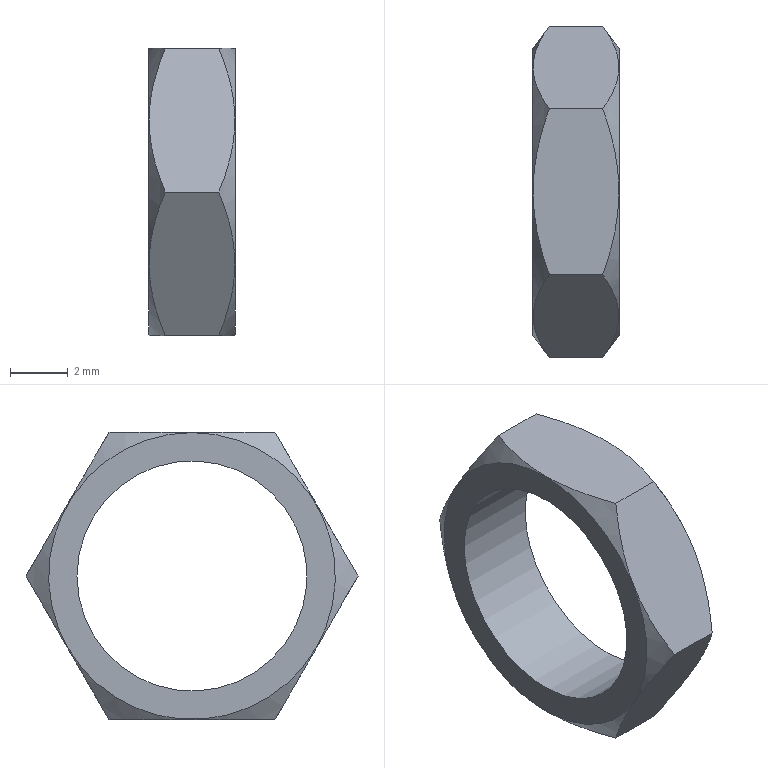Part | STEP file | 1-43.15 | 1 solid | 11 faces | box 3 x 11.547 x 10 mm | volume 106.106 mm3 | plane 8 | cone 2 | cylinder 1 | commonest cylinder face diameters 8 x1
STEP:
#1=CARTESIAN_POINT('',(0.,0.,0.));
#2=DIRECTION('',(0.,0.,1.));
#3=DIRECTION('',(1.,0.,0.));
#4=AXIS2_PLACEMENT_3D('',#1,#2,#3);
#5=CARTESIAN_POINT('',(1.5,4.,0.));
#6=VERTEX_POINT('',#5);
#7=CARTESIAN_POINT('',(1.5,0.,0.));
#8=DIRECTION('',(-1.,0.,0.));
#9=DIRECTION('',(0.,1.,0.));
#10=AXIS2_PLACEMENT_3D('',#7,#8,#9);
#11=CIRCLE('',#10,4.);
#12=CARTESIAN_POINT('',(1.5,0.,0.));
#13=DIRECTION('',(-1.,0.,0.));
#14=DIRECTION('',(0.,1.,0.));
#15=AXIS2_PLACEMENT_3D('',#12,#13,#14);
#16=CYLINDRICAL_SURFACE('',#15,4.);
#17=CARTESIAN_POINT('',(0.,0.));
#18=DIRECTION('',(1.,0.));
#19=VECTOR('',#18,1.);
#20=LINE('',#17,#19);
#21=(GEOMETRIC_REPRESENTATION_CONTEXT(2)PARAMETRIC_REPRESENTATION_CONTEXT()REPRESENTATION_CONTEXT('',''));
#22=DEFINITIONAL_REPRESENTATION('',(#20),#21);
#23=PCURVE('',#16,#22);
#24=CARTESIAN_POINT('',(1.5,0.,0.7735));
#25=DIRECTION('',(1.,0.,0.));
#26=DIRECTION('',(0.,1.,0.));
#27=AXIS2_PLACEMENT_3D('',#24,#25,#26);
#28=PLANE('',#27);
#29=CARTESIAN_POINT('',(4.,-0.7735));
#30=CARTESIAN_POINT('',(4.,-7.702));
#31=CARTESIAN_POINT('',(-2.,-4.238));
#32=CARTESIAN_POINT('',(-8.,-0.7735));
#33=CARTESIAN_POINT('',(-2.,2.691));
#34=CARTESIAN_POINT('',(4.,6.155));
#35=CARTESIAN_POINT('',(4.,-0.7735));
#36=(BOUNDED_CURVE()B_SPLINE_CURVE(2,(#29,#30,#31,#32,#33,#34,#35),.UNSPECIFIED.,.T.,.F.)B_SPLINE_CURVE_WITH_KNOTS((1,2,2,2,2,1),(-2.094,0.,2.094,4.189,6.283,8.378),.UNSPECIFIED.)CURVE()GEOMETRIC_REPRESENTATION_ITEM()RATIONAL_B_SPLINE_CURVE((1.,0.5,1.,0.5,1.,0.5,1.))REPRESENTATION_ITEM(''));
#37=(GEOMETRIC_REPRESENTATION_CONTEXT(2)PARAMETRIC_REPRESENTATION_CONTEXT()REPRESENTATION_CONTEXT('',''));
#38=DEFINITIONAL_REPRESENTATION('',(#36),#37);
#39=PCURVE('',#28,#38);
#40=SURFACE_CURVE('',#11,(#23,#39),.PCURVE_S1.);
#41=EDGE_CURVE('',#6,#6,#40,.T.);
#42=ORIENTED_EDGE('',*,*,#41,.T.);
#43=CARTESIAN_POINT('',(-1.5,4.,0.));
#44=VERTEX_POINT('',#43);
#45=CARTESIAN_POINT('',(1.5,4.,0.));
#46=DIRECTION('',(-1.,0.,0.));
#47=VECTOR('',#46,1.);
#48=LINE('',#45,#47);
#49=CARTESIAN_POINT('',(6.283,0.));
#50=DIRECTION('',(0.,1.));
#51=VECTOR('',#50,1.);
#52=LINE('',#49,#51);
#53=(GEOMETRIC_REPRESENTATION_CONTEXT(2)PARAMETRIC_REPRESENTATION_CONTEXT()REPRESENTATION_CONTEXT('',''));
#54=DEFINITIONAL_REPRESENTATION('',(#52),#53);
#55=PCURVE('',#16,#54);
#56=CARTESIAN_POINT('',(0.,0.));
#57=DIRECTION('',(0.,1.));
#58=VECTOR('',#57,1.);
#59=LINE('',#56,#58);
#60=(GEOMETRIC_REPRESENTATION_CONTEXT(2)PARAMETRIC_REPRESENTATION_CONTEXT()REPRESENTATION_CONTEXT('',''));
#61=DEFINITIONAL_REPRESENTATION('',(#59),#60);
#62=PCURVE('',#16,#61);
#63=SEAM_CURVE('',#48,(#55,#62),.PCURVE_S1.);
#64=EDGE_CURVE('',#6,#44,#63,.T.);
#65=ORIENTED_EDGE('',*,*,#64,.T.);
#66=CARTESIAN_POINT('',(-1.5,0.,0.));
#67=DIRECTION('',(-1.,0.,0.));
#68=DIRECTION('',(0.,1.,0.));
#69=AXIS2_PLACEMENT_3D('',#66,#67,#68);
#70=CIRCLE('',#69,4.);
#71=CARTESIAN_POINT('',(0.,3.));
#72=DIRECTION('',(1.,0.));
#73=VECTOR('',#72,1.);
#74=LINE('',#71,#73);
#75=(GEOMETRIC_REPRESENTATION_CONTEXT(2)PARAMETRIC_REPRESENTATION_CONTEXT()REPRESENTATION_CONTEXT('',''));
#76=DEFINITIONAL_REPRESENTATION('',(#74),#75);
#77=PCURVE('',#16,#76);
#78=CARTESIAN_POINT('',(-1.5,0.,0.7735));
#79=DIRECTION('',(1.,0.,0.));
#80=DIRECTION('',(0.,1.,0.));
#81=AXIS2_PLACEMENT_3D('',#78,#79,#80);
#82=PLANE('',#81);
#83=CARTESIAN_POINT('',(4.,-0.7735));
#84=CARTESIAN_POINT('',(4.,-7.702));
#85=CARTESIAN_POINT('',(-2.,-4.238));
#86=CARTESIAN_POINT('',(-8.,-0.7735));
#87=CARTESIAN_POINT('',(-2.,2.691));
#88=CARTESIAN_POINT('',(4.,6.155));
#89=CARTESIAN_POINT('',(4.,-0.7735));
#90=(BOUNDED_CURVE()B_SPLINE_CURVE(2,(#83,#84,#85,#86,#87,#88,#89),.UNSPECIFIED.,.T.,.F.)B_SPLINE_CURVE_WITH_KNOTS((1,2,2,2,2,1),(-2.094,0.,2.094,4.189,6.283,8.378),.UNSPECIFIED.)CURVE()GEOMETRIC_REPRESENTATION_ITEM()RATIONAL_B_SPLINE_CURVE((1.,0.5,1.,0.5,1.,0.5,1.))REPRESENTATION_ITEM(''));
#91=(GEOMETRIC_REPRESENTATION_CONTEXT(2)PARAMETRIC_REPRESENTATION_CONTEXT()REPRESENTATION_CONTEXT('',''));
#92=DEFINITIONAL_REPRESENTATION('',(#90),#91);
#93=PCURVE('',#82,#92);
#94=SURFACE_CURVE('',#70,(#77,#93),.PCURVE_S1.);
#95=EDGE_CURVE('',#44,#44,#94,.T.);
#96=ORIENTED_EDGE('',*,*,#95,.F.);
#97=ORIENTED_EDGE('',*,*,#64,.F.);
#98=EDGE_LOOP('',(#42,#65,#96,#97));
#99=FACE_BOUND('',#98,.F.);
#100=ADVANCED_FACE('',(#99),#16,.F.);
#101=CARTESIAN_POINT('',(1.5,0.,4.986));
#102=VERTEX_POINT('',#101);
#103=CARTESIAN_POINT('',(1.5,0.,0.));
#104=DIRECTION('',(1.,0.,0.));
#105=DIRECTION('',(0.,0.,1.));
#106=AXIS2_PLACEMENT_3D('',#103,#104,#105);
#107=CIRCLE('',#106,4.986);
#108=CARTESIAN_POINT('',(0.,-0.7735));
#109=DIRECTION('',(0.,1.));
#110=AXIS2_PLACEMENT_2D('',#108,#109);
#111=CIRCLE('',#110,4.986);
#112=(GEOMETRIC_REPRESENTATION_CONTEXT(2)PARAMETRIC_REPRESENTATION_CONTEXT()REPRESENTATION_CONTEXT('',''));
#113=DEFINITIONAL_REPRESENTATION('',(#111),#112);
#114=PCURVE('',#28,#113);
#115=CARTESIAN_POINT('',(1.5,0.,0.));
#116=DIRECTION('',(-1.,0.,0.));
#117=DIRECTION('',(0.,0.,1.));
#118=AXIS2_PLACEMENT_3D('',#115,#116,#117);
#119=CONICAL_SURFACE('',#118,4.986,0.9416);
#120=CARTESIAN_POINT('',(6.283,0.));
#121=DIRECTION('',(-1.,0.));
#122=VECTOR('',#121,1.);
#123=LINE('',#120,#122);
#124=(GEOMETRIC_REPRESENTATION_CONTEXT(2)PARAMETRIC_REPRESENTATION_CONTEXT()REPRESENTATION_CONTEXT('',''));
#125=DEFINITIONAL_REPRESENTATION('',(#123),#124);
#126=PCURVE('',#119,#125);
#127=SURFACE_CURVE('',#107,(#114,#126),.PCURVE_S1.);
#128=EDGE_CURVE('',#102,#102,#127,.T.);
#129=ORIENTED_EDGE('',*,*,#128,.T.);
#130=EDGE_LOOP('',(#129));
#131=FACE_BOUND('',#130,.T.);
#132=ORIENTED_EDGE('',*,*,#41,.T.);
#133=EDGE_LOOP('',(#132));
#134=FACE_BOUND('',#133,.T.);
#135=ADVANCED_FACE('',(#131,#134),#28,.T.);
#136=CARTESIAN_POINT('',(-1.5,0.,4.986));
#137=VERTEX_POINT('',#136);
#138=CARTESIAN_POINT('',(-1.5,0.,0.));
#139=DIRECTION('',(1.,0.,0.));
#140=DIRECTION('',(0.,0.,1.));
#141=AXIS2_PLACEMENT_3D('',#138,#139,#140);
#142=CIRCLE('',#141,4.986);
#143=CARTESIAN_POINT('',(0.,-0.7735));
#144=DIRECTION('',(0.,1.));
#145=AXIS2_PLACEMENT_2D('',#143,#144);
#146=CIRCLE('',#145,4.986);
#147=(GEOMETRIC_REPRESENTATION_CONTEXT(2)PARAMETRIC_REPRESENTATION_CONTEXT()REPRESENTATION_CONTEXT('',''));
#148=DEFINITIONAL_REPRESENTATION('',(#146),#147);
#149=PCURVE('',#82,#148);
#150=CARTESIAN_POINT('',(-1.5,0.,0.));
#151=DIRECTION('',(1.,0.,0.));
#152=DIRECTION('',(0.,0.,1.));
#153=AXIS2_PLACEMENT_3D('',#150,#151,#152);
#154=CONICAL_SURFACE('',#153,4.986,0.9416);
#155=CARTESIAN_POINT('',(0.,0.));
#156=DIRECTION('',(1.,0.));
#157=VECTOR('',#156,1.);
#158=LINE('',#155,#157);
#159=(GEOMETRIC_REPRESENTATION_CONTEXT(2)PARAMETRIC_REPRESENTATION_CONTEXT()REPRESENTATION_CONTEXT('',''));
#160=DEFINITIONAL_REPRESENTATION('',(#158),#159);
#161=PCURVE('',#154,#160);
#162=SURFACE_CURVE('',#142,(#149,#161),.PCURVE_S1.);
#163=EDGE_CURVE('',#137,#137,#162,.T.);
#164=ORIENTED_EDGE('',*,*,#163,.T.);
#165=EDGE_LOOP('',(#164));
#166=FACE_BOUND('',#165,.F.);
#167=ORIENTED_EDGE('',*,*,#95,.T.);
#168=EDGE_LOOP('',(#167));
#169=FACE_BOUND('',#168,.F.);
#170=ADVANCED_FACE('',(#166,#169),#82,.F.);
#171=CARTESIAN_POINT('',(0.9268,5.774,0.));
#172=VERTEX_POINT('',#171);
#173=CARTESIAN_POINT('',(-0.9268,5.774,0.));
#174=VERTEX_POINT('',#173);
#175=CARTESIAN_POINT('',(0.9268,5.774,0.));
#176=DIRECTION('',(-1.,0.,0.));
#177=VECTOR('',#176,1.);
#178=LINE('',#175,#177);
#179=CARTESIAN_POINT('',(0.,4.33,2.5));
#180=DIRECTION('',(0.,-0.866,-0.5));
#181=DIRECTION('',(0.,-0.5,0.866));
#182=AXIS2_PLACEMENT_3D('',#179,#180,#181);
#183=PLANE('',#182);
#184=CARTESIAN_POINT('',(-2.887,-0.9268));
#185=DIRECTION('',(0.,1.));
#186=VECTOR('',#185,1.);
#187=LINE('',#184,#186);
#188=(GEOMETRIC_REPRESENTATION_CONTEXT(2)PARAMETRIC_REPRESENTATION_CONTEXT()REPRESENTATION_CONTEXT('',''));
#189=DEFINITIONAL_REPRESENTATION('',(#187),#188);
#190=PCURVE('',#183,#189);
#191=CARTESIAN_POINT('',(0.,4.33,-2.5));
#192=DIRECTION('',(0.,-0.866,0.5));
#193=DIRECTION('',(0.,0.5,0.866));
#194=AXIS2_PLACEMENT_3D('',#191,#192,#193);
#195=PLANE('',#194);
#196=CARTESIAN_POINT('',(2.887,-0.9268));
#197=DIRECTION('',(0.,1.));
#198=VECTOR('',#197,1.);
#199=LINE('',#196,#198);
#200=(GEOMETRIC_REPRESENTATION_CONTEXT(2)PARAMETRIC_REPRESENTATION_CONTEXT()REPRESENTATION_CONTEXT('',''));
#201=DEFINITIONAL_REPRESENTATION('',(#199),#200);
#202=PCURVE('',#195,#201);
#203=SURFACE_CURVE('',#178,(#190,#202),.PCURVE_S1.);
#204=EDGE_CURVE('',#172,#174,#203,.T.);
#205=ORIENTED_EDGE('',*,*,#204,.F.);
#206=CARTESIAN_POINT('',(0.9268,2.887,5.));
#207=VERTEX_POINT('',#206);
#208=CARTESIAN_POINT('',(0.9268,5.774,0.));
#209=CARTESIAN_POINT('',(1.977,4.33,2.5));
#210=CARTESIAN_POINT('',(0.9268,2.887,5.));
#211=(BOUNDED_CURVE()B_SPLINE_CURVE(2,(#208,#209,#210),.UNSPECIFIED.,.F.,.F.)B_SPLINE_CURVE_WITH_KNOTS((3,3),(0.,1.),.PIECEWISE_BEZIER_KNOTS.)CURVE()GEOMETRIC_REPRESENTATION_ITEM()RATIONAL_B_SPLINE_CURVE((1.118,1.291,1.118))REPRESENTATION_ITEM(''));
#212=CARTESIAN_POINT('',(-2.887,-0.9268));
#213=CARTESIAN_POINT('',(0.,-1.977));
#214=CARTESIAN_POINT('',(2.887,-0.9268));
#215=(BOUNDED_CURVE()B_SPLINE_CURVE(2,(#212,#213,#214),.UNSPECIFIED.,.F.,.F.)B_SPLINE_CURVE_WITH_KNOTS((3,3),(0.,1.),.PIECEWISE_BEZIER_KNOTS.)CURVE()GEOMETRIC_REPRESENTATION_ITEM()RATIONAL_B_SPLINE_CURVE((1.118,1.291,1.118))REPRESENTATION_ITEM(''));
#216=(GEOMETRIC_REPRESENTATION_CONTEXT(2)PARAMETRIC_REPRESENTATION_CONTEXT()REPRESENTATION_CONTEXT('',''));
#217=DEFINITIONAL_REPRESENTATION('',(#215),#216);
#218=PCURVE('',#183,#217);
#219=CARTESIAN_POINT('',(1.571,0.5732));
#220=CARTESIAN_POINT('',(1.556,0.5365));
#221=CARTESIAN_POINT('',(1.525,0.4673));
#222=CARTESIAN_POINT('',(1.479,0.3758));
#223=CARTESIAN_POINT('',(1.432,0.2957));
#224=CARTESIAN_POINT('',(1.385,0.2264));
#225=CARTESIAN_POINT('',(1.338,0.1674));
#226=CARTESIAN_POINT('',(1.29,0.1182));
#227=CARTESIAN_POINT('',(1.241,0.0784));
#228=CARTESIAN_POINT('',(1.193,0.04775));
#229=CARTESIAN_POINT('',(1.145,0.02601));
#230=CARTESIAN_POINT('',(1.096,0.01303));
#231=CARTESIAN_POINT('',(1.047,0.008712));
#232=CARTESIAN_POINT('',(0.9985,0.01303));
#233=CARTESIAN_POINT('',(0.9498,0.02601));
#234=CARTESIAN_POINT('',(0.9013,0.04775));
#235=CARTESIAN_POINT('',(0.8529,0.0784));
#236=CARTESIAN_POINT('',(0.8048,0.1182));
#237=CARTESIAN_POINT('',(0.7569,0.1674));
#238=CARTESIAN_POINT('',(0.7094,0.2264));
#239=CARTESIAN_POINT('',(0.6622,0.2957));
#240=CARTESIAN_POINT('',(0.6155,0.3758));
#241=CARTESIAN_POINT('',(0.5692,0.4673));
#242=CARTESIAN_POINT('',(0.5388,0.5365));
#243=CARTESIAN_POINT('',(0.5236,0.5732));
#244=B_SPLINE_CURVE_WITH_KNOTS('',3,(#219,#220,#221,#222,#223,#224,#225,#226,#227,#228,#229,#230,#231,#232,#233,#234,#235,#236,#237,#238,#239,#240,#241,#242,#243),.UNSPECIFIED.,.F.,.F.,(4,1,1,1,1,1,1,1,1,1,1,1,1,1,1,1,1,1,1,1,1,1,4),(0.,0.04545,0.09091,0.1364,0.1818,0.2273,0.2727,0.3182,0.3636,0.4091,0.4545,0.5,0.5455,0.5909,0.6364,0.6818,0.7273,0.7727,0.8182,0.8636,0.9091,0.9545,1.),.QUASI_UNIFORM_KNOTS.);
#245=(GEOMETRIC_REPRESENTATION_CONTEXT(2)PARAMETRIC_REPRESENTATION_CONTEXT()REPRESENTATION_CONTEXT('',''));
#246=DEFINITIONAL_REPRESENTATION('',(#244),#245);
#247=PCURVE('',#119,#246);
#248=SURFACE_CURVE('',#211,(#218,#247),.PCURVE_S1.);
#249=EDGE_CURVE('',#172,#207,#248,.T.);
#250=ORIENTED_EDGE('',*,*,#249,.T.);
#251=CARTESIAN_POINT('',(-0.9268,2.887,5.));
#252=VERTEX_POINT('',#251);
#253=CARTESIAN_POINT('',(0.9268,2.887,5.));
#254=DIRECTION('',(-1.,0.,0.));
#255=VECTOR('',#254,1.);
#256=LINE('',#253,#255);
#257=CARTESIAN_POINT('',(2.887,-0.9268));
#258=DIRECTION('',(0.,1.));
#259=VECTOR('',#258,1.);
#260=LINE('',#257,#259);
#261=(GEOMETRIC_REPRESENTATION_CONTEXT(2)PARAMETRIC_REPRESENTATION_CONTEXT()REPRESENTATION_CONTEXT('',''));
#262=DEFINITIONAL_REPRESENTATION('',(#260),#261);
#263=PCURVE('',#183,#262);
#264=CARTESIAN_POINT('',(0.,0.,5.));
#265=DIRECTION('',(0.,0.,-1.));
#266=DIRECTION('',(0.,-1.,0.));
#267=AXIS2_PLACEMENT_3D('',#264,#265,#266);
#268=PLANE('',#267);
#269=CARTESIAN_POINT('',(-2.887,-0.9268));
#270=DIRECTION('',(0.,1.));
#271=VECTOR('',#270,1.);
#272=LINE('',#269,#271);
#273=(GEOMETRIC_REPRESENTATION_CONTEXT(2)PARAMETRIC_REPRESENTATION_CONTEXT()REPRESENTATION_CONTEXT('',''));
#274=DEFINITIONAL_REPRESENTATION('',(#272),#273);
#275=PCURVE('',#268,#274);
#276=SURFACE_CURVE('',#256,(#263,#275),.PCURVE_S1.);
#277=EDGE_CURVE('',#207,#252,#276,.T.);
#278=ORIENTED_EDGE('',*,*,#277,.T.);
#279=CARTESIAN_POINT('',(-0.9268,2.887,5.));
#280=CARTESIAN_POINT('',(-1.977,4.33,2.5));
#281=CARTESIAN_POINT('',(-0.9268,5.774,0.));
#282=(BOUNDED_CURVE()B_SPLINE_CURVE(2,(#279,#280,#281),.UNSPECIFIED.,.F.,.F.)B_SPLINE_CURVE_WITH_KNOTS((3,3),(0.,1.),.PIECEWISE_BEZIER_KNOTS.)CURVE()GEOMETRIC_REPRESENTATION_ITEM()RATIONAL_B_SPLINE_CURVE((1.118,1.291,1.118))REPRESENTATION_ITEM(''));
#283=CARTESIAN_POINT('',(2.887,0.9268));
#284=CARTESIAN_POINT('',(0.,1.977));
#285=CARTESIAN_POINT('',(-2.887,0.9268));
#286=(BOUNDED_CURVE()B_SPLINE_CURVE(2,(#283,#284,#285),.UNSPECIFIED.,.F.,.F.)B_SPLINE_CURVE_WITH_KNOTS((3,3),(0.,1.),.PIECEWISE_BEZIER_KNOTS.)CURVE()GEOMETRIC_REPRESENTATION_ITEM()RATIONAL_B_SPLINE_CURVE((1.118,1.291,1.118))REPRESENTATION_ITEM(''));
#287=(GEOMETRIC_REPRESENTATION_CONTEXT(2)PARAMETRIC_REPRESENTATION_CONTEXT()REPRESENTATION_CONTEXT('',''));
#288=DEFINITIONAL_REPRESENTATION('',(#286),#287);
#289=PCURVE('',#183,#288);
#290=CARTESIAN_POINT('',(5.76,0.5732));
#291=CARTESIAN_POINT('',(5.744,0.5365));
#292=CARTESIAN_POINT('',(5.714,0.4673));
#293=CARTESIAN_POINT('',(5.668,0.3758));
#294=CARTESIAN_POINT('',(5.621,0.2957));
#295=CARTESIAN_POINT('',(5.574,0.2264));
#296=CARTESIAN_POINT('',(5.526,0.1674));
#297=CARTESIAN_POINT('',(5.478,0.1182));
#298=CARTESIAN_POINT('',(5.43,0.0784));
#299=CARTESIAN_POINT('',(5.382,0.04775));
#300=CARTESIAN_POINT('',(5.333,0.02601));
#301=CARTESIAN_POINT('',(5.285,0.01303));
#302=CARTESIAN_POINT('',(5.236,0.008712));
#303=CARTESIAN_POINT('',(5.187,0.01303));
#304=CARTESIAN_POINT('',(5.139,0.02601));
#305=CARTESIAN_POINT('',(5.09,0.04775));
#306=CARTESIAN_POINT('',(5.042,0.0784));
#307=CARTESIAN_POINT('',(4.994,0.1182));
#308=CARTESIAN_POINT('',(4.946,0.1674));
#309=CARTESIAN_POINT('',(4.898,0.2264));
#310=CARTESIAN_POINT('',(4.851,0.2957));
#311=CARTESIAN_POINT('',(4.804,0.3758));
#312=CARTESIAN_POINT('',(4.758,0.4673));
#313=CARTESIAN_POINT('',(4.728,0.5365));
#314=CARTESIAN_POINT('',(4.712,0.5732));
#315=B_SPLINE_CURVE_WITH_KNOTS('',3,(#290,#291,#292,#293,#294,#295,#296,#297,#298,#299,#300,#301,#302,#303,#304,#305,#306,#307,#308,#309,#310,#311,#312,#313,#314),.UNSPECIFIED.,.F.,.F.,(4,1,1,1,1,1,1,1,1,1,1,1,1,1,1,1,1,1,1,1,1,1,4),(0.,0.04545,0.09091,0.1364,0.1818,0.2273,0.2727,0.3182,0.3636,0.4091,0.4545,0.5,0.5455,0.5909,0.6364,0.6818,0.7273,0.7727,0.8182,0.8636,0.9091,0.9545,1.),.QUASI_UNIFORM_KNOTS.);
#316=(GEOMETRIC_REPRESENTATION_CONTEXT(2)PARAMETRIC_REPRESENTATION_CONTEXT()REPRESENTATION_CONTEXT('',''));
#317=DEFINITIONAL_REPRESENTATION('',(#315),#316);
#318=PCURVE('',#154,#317);
#319=SURFACE_CURVE('',#282,(#289,#318),.PCURVE_S1.);
#320=EDGE_CURVE('',#252,#174,#319,.T.);
#321=ORIENTED_EDGE('',*,*,#320,.T.);
#322=EDGE_LOOP('',(#205,#250,#278,#321));
#323=FACE_BOUND('',#322,.F.);
#324=ADVANCED_FACE('',(#323),#183,.F.);
#325=ORIENTED_EDGE('',*,*,#277,.F.);
#326=CARTESIAN_POINT('',(1.49,0.,5.));
#327=VERTEX_POINT('',#326);
#328=CARTESIAN_POINT('',(0.9268,2.887,5.));
#329=CARTESIAN_POINT('',(1.49,1.34,5.));
#330=CARTESIAN_POINT('',(1.49,0.,5.));
#331=(BOUNDED_CURVE()B_SPLINE_CURVE(2,(#328,#329,#330),.UNSPECIFIED.,.F.,.F.)B_SPLINE_CURVE_WITH_KNOTS((3,3),(0.,1.),.PIECEWISE_BEZIER_KNOTS.)CURVE()GEOMETRIC_REPRESENTATION_ITEM()RATIONAL_B_SPLINE_CURVE((1.118,1.205,1.205))REPRESENTATION_ITEM(''));
#332=CARTESIAN_POINT('',(-2.887,-0.9268));
#333=CARTESIAN_POINT('',(-1.34,-1.49));
#334=CARTESIAN_POINT('',(0.,-1.49));
#335=(BOUNDED_CURVE()B_SPLINE_CURVE(2,(#332,#333,#334),.UNSPECIFIED.,.F.,.F.)B_SPLINE_CURVE_WITH_KNOTS((3,3),(0.,1.),.PIECEWISE_BEZIER_KNOTS.)CURVE()GEOMETRIC_REPRESENTATION_ITEM()RATIONAL_B_SPLINE_CURVE((1.118,1.205,1.205))REPRESENTATION_ITEM(''));
#336=(GEOMETRIC_REPRESENTATION_CONTEXT(2)PARAMETRIC_REPRESENTATION_CONTEXT()REPRESENTATION_CONTEXT('',''));
#337=DEFINITIONAL_REPRESENTATION('',(#335),#336);
#338=PCURVE('',#268,#337);
#339=CARTESIAN_POINT('',(0.5236,0.5732));
#340=CARTESIAN_POINT('',(0.516,0.5548));
#341=CARTESIAN_POINT('',(0.5008,0.5192));
#342=CARTESIAN_POINT('',(0.4779,0.4688));
#343=CARTESIAN_POINT('',(0.4548,0.4215));
#344=CARTESIAN_POINT('',(0.4317,0.3772));
#345=CARTESIAN_POINT('',(0.4084,0.3357));
#346=CARTESIAN_POINT('',(0.3849,0.297));
#347=CARTESIAN_POINT('',(0.3614,0.2611));
#348=CARTESIAN_POINT('',(0.3378,0.2277));
#349=CARTESIAN_POINT('',(0.3141,0.1969));
#350=CARTESIAN_POINT('',(0.2903,0.1686));
#351=CARTESIAN_POINT('',(0.2664,0.1428));
#352=CARTESIAN_POINT('',(0.2424,0.1194));
#353=CARTESIAN_POINT('',(0.2184,0.09829));
#354=CARTESIAN_POINT('',(0.1943,0.07954));
#355=CARTESIAN_POINT('',(0.1701,0.06307));
#356=CARTESIAN_POINT('',(0.1459,0.04886));
#357=CARTESIAN_POINT('',(0.1217,0.03688));
#358=CARTESIAN_POINT('',(0.09736,0.0271));
#359=CARTESIAN_POINT('',(0.07305,0.01952));
#360=CARTESIAN_POINT('',(0.04871,0.01411));
#361=CARTESIAN_POINT('',(0.02436,0.01087));
#362=CARTESIAN_POINT('',(0.00812,0.01015));
#363=CARTESIAN_POINT('',(0.,0.01015));
#364=B_SPLINE_CURVE_WITH_KNOTS('',3,(#339,#340,#341,#342,#343,#344,#345,#346,#347,#348,#349,#350,#351,#352,#353,#354,#355,#356,#357,#358,#359,#360,#361,#362,#363),.UNSPECIFIED.,.F.,.F.,(4,1,1,1,1,1,1,1,1,1,1,1,1,1,1,1,1,1,1,1,1,1,4),(0.,0.04545,0.09091,0.1364,0.1818,0.2273,0.2727,0.3182,0.3636,0.4091,0.4545,0.5,0.5455,0.5909,0.6364,0.6818,0.7273,0.7727,0.8182,0.8636,0.9091,0.9545,1.),.QUASI_UNIFORM_KNOTS.);
#365=(GEOMETRIC_REPRESENTATION_CONTEXT(2)PARAMETRIC_REPRESENTATION_CONTEXT()REPRESENTATION_CONTEXT('',''));
#366=DEFINITIONAL_REPRESENTATION('',(#364),#365);
#367=PCURVE('',#119,#366);
#368=SURFACE_CURVE('',#331,(#338,#367),.PCURVE_S1.);
#369=EDGE_CURVE('',#207,#327,#368,.T.);
#370=ORIENTED_EDGE('',*,*,#369,.T.);
#371=CARTESIAN_POINT('',(0.9268,-2.887,5.));
#372=VERTEX_POINT('',#371);
#373=CARTESIAN_POINT('',(1.49,0.,5.));
#374=CARTESIAN_POINT('',(1.49,-1.34,5.));
#375=CARTESIAN_POINT('',(0.9268,-2.887,5.));
#376=(BOUNDED_CURVE()B_SPLINE_CURVE(2,(#373,#374,#375),.UNSPECIFIED.,.F.,.F.)B_SPLINE_CURVE_WITH_KNOTS((3,3),(0.,1.),.PIECEWISE_BEZIER_KNOTS.)CURVE()GEOMETRIC_REPRESENTATION_ITEM()RATIONAL_B_SPLINE_CURVE((1.205,1.205,1.118))REPRESENTATION_ITEM(''));
#377=CARTESIAN_POINT('',(0.,-1.49));
#378=CARTESIAN_POINT('',(1.34,-1.49));
#379=CARTESIAN_POINT('',(2.887,-0.9268));
#380=(BOUNDED_CURVE()B_SPLINE_CURVE(2,(#377,#378,#379),.UNSPECIFIED.,.F.,.F.)B_SPLINE_CURVE_WITH_KNOTS((3,3),(0.,1.),.PIECEWISE_BEZIER_KNOTS.)CURVE()GEOMETRIC_REPRESENTATION_ITEM()RATIONAL_B_SPLINE_CURVE((1.205,1.205,1.118))REPRESENTATION_ITEM(''));
#381=(GEOMETRIC_REPRESENTATION_CONTEXT(2)PARAMETRIC_REPRESENTATION_CONTEXT()REPRESENTATION_CONTEXT('',''));
#382=DEFINITIONAL_REPRESENTATION('',(#380),#381);
#383=PCURVE('',#268,#382);
#384=CARTESIAN_POINT('',(6.283,0.01015));
#385=CARTESIAN_POINT('',(6.275,0.01015));
#386=CARTESIAN_POINT('',(6.259,0.01087));
#387=CARTESIAN_POINT('',(6.234,0.01411));
#388=CARTESIAN_POINT('',(6.21,0.01952));
#389=CARTESIAN_POINT('',(6.186,0.0271));
#390=CARTESIAN_POINT('',(6.162,0.03688));
#391=CARTESIAN_POINT('',(6.137,0.04886));
#392=CARTESIAN_POINT('',(6.113,0.06307));
#393=CARTESIAN_POINT('',(6.089,0.07954));
#394=CARTESIAN_POINT('',(6.065,0.09829));
#395=CARTESIAN_POINT('',(6.041,0.1194));
#396=CARTESIAN_POINT('',(6.017,0.1428));
#397=CARTESIAN_POINT('',(5.993,0.1686));
#398=CARTESIAN_POINT('',(5.969,0.1969));
#399=CARTESIAN_POINT('',(5.945,0.2277));
#400=CARTESIAN_POINT('',(5.922,0.2611));
#401=CARTESIAN_POINT('',(5.898,0.297));
#402=CARTESIAN_POINT('',(5.875,0.3357));
#403=CARTESIAN_POINT('',(5.852,0.3772));
#404=CARTESIAN_POINT('',(5.828,0.4215));
#405=CARTESIAN_POINT('',(5.805,0.4688));
#406=CARTESIAN_POINT('',(5.782,0.5192));
#407=CARTESIAN_POINT('',(5.767,0.5548));
#408=CARTESIAN_POINT('',(5.76,0.5732));
#409=B_SPLINE_CURVE_WITH_KNOTS('',3,(#384,#385,#386,#387,#388,#389,#390,#391,#392,#393,#394,#395,#396,#397,#398,#399,#400,#401,#402,#403,#404,#405,#406,#407,#408),.UNSPECIFIED.,.F.,.F.,(4,1,1,1,1,1,1,1,1,1,1,1,1,1,1,1,1,1,1,1,1,1,4),(0.,0.04545,0.09091,0.1364,0.1818,0.2273,0.2727,0.3182,0.3636,0.4091,0.4545,0.5,0.5455,0.5909,0.6364,0.6818,0.7273,0.7727,0.8182,0.8636,0.9091,0.9545,1.),.QUASI_UNIFORM_KNOTS.);
#410=(GEOMETRIC_REPRESENTATION_CONTEXT(2)PARAMETRIC_REPRESENTATION_CONTEXT()REPRESENTATION_CONTEXT('',''));
#411=DEFINITIONAL_REPRESENTATION('',(#409),#410);
#412=PCURVE('',#119,#411);
#413=SURFACE_CURVE('',#376,(#383,#412),.PCURVE_S1.);
#414=EDGE_CURVE('',#327,#372,#413,.T.);
#415=ORIENTED_EDGE('',*,*,#414,.T.);
#416=CARTESIAN_POINT('',(-0.9268,-2.887,5.));
#417=VERTEX_POINT('',#416);
#418=CARTESIAN_POINT('',(0.9268,-2.887,5.));
#419=DIRECTION('',(-1.,0.,0.));
#420=VECTOR('',#419,1.);
#421=LINE('',#418,#420);
#422=CARTESIAN_POINT('',(2.887,-0.9268));
#423=DIRECTION('',(0.,1.));
#424=VECTOR('',#423,1.);
#425=LINE('',#422,#424);
#426=(GEOMETRIC_REPRESENTATION_CONTEXT(2)PARAMETRIC_REPRESENTATION_CONTEXT()REPRESENTATION_CONTEXT('',''));
#427=DEFINITIONAL_REPRESENTATION('',(#425),#426);
#428=PCURVE('',#268,#427);
#429=CARTESIAN_POINT('',(0.,-4.33,2.5));
#430=DIRECTION('',(0.,0.866,-0.5));
#431=DIRECTION('',(0.,-0.5,-0.866));
#432=AXIS2_PLACEMENT_3D('',#429,#430,#431);
#433=PLANE('',#432);
#434=CARTESIAN_POINT('',(-2.887,-0.9268));
#435=DIRECTION('',(0.,1.));
#436=VECTOR('',#435,1.);
#437=LINE('',#434,#436);
#438=(GEOMETRIC_REPRESENTATION_CONTEXT(2)PARAMETRIC_REPRESENTATION_CONTEXT()REPRESENTATION_CONTEXT('',''));
#439=DEFINITIONAL_REPRESENTATION('',(#437),#438);
#440=PCURVE('',#433,#439);
#441=SURFACE_CURVE('',#421,(#428,#440),.PCURVE_S1.);
#442=EDGE_CURVE('',#372,#417,#441,.T.);
#443=ORIENTED_EDGE('',*,*,#442,.T.);
#444=CARTESIAN_POINT('',(-1.49,0.,5.));
#445=VERTEX_POINT('',#444);
#446=CARTESIAN_POINT('',(-0.9268,-2.887,5.));
#447=CARTESIAN_POINT('',(-1.49,-1.34,5.));
#448=CARTESIAN_POINT('',(-1.49,0.,5.));
#449=(BOUNDED_CURVE()B_SPLINE_CURVE(2,(#446,#447,#448),.UNSPECIFIED.,.F.,.F.)B_SPLINE_CURVE_WITH_KNOTS((3,3),(0.,1.),.PIECEWISE_BEZIER_KNOTS.)CURVE()GEOMETRIC_REPRESENTATION_ITEM()RATIONAL_B_SPLINE_CURVE((1.118,1.205,1.205))REPRESENTATION_ITEM(''));
#450=CARTESIAN_POINT('',(2.887,0.9268));
#451=CARTESIAN_POINT('',(1.34,1.49));
#452=CARTESIAN_POINT('',(0.,1.49));
#453=(BOUNDED_CURVE()B_SPLINE_CURVE(2,(#450,#451,#452),.UNSPECIFIED.,.F.,.F.)B_SPLINE_CURVE_WITH_KNOTS((3,3),(0.,1.),.PIECEWISE_BEZIER_KNOTS.)CURVE()GEOMETRIC_REPRESENTATION_ITEM()RATIONAL_B_SPLINE_CURVE((1.118,1.205,1.205))REPRESENTATION_ITEM(''));
#454=(GEOMETRIC_REPRESENTATION_CONTEXT(2)PARAMETRIC_REPRESENTATION_CONTEXT()REPRESENTATION_CONTEXT('',''));
#455=DEFINITIONAL_REPRESENTATION('',(#453),#454);
#456=PCURVE('',#268,#455);
#457=CARTESIAN_POINT('',(0.5236,0.5732));
#458=CARTESIAN_POINT('',(0.516,0.5548));
#459=CARTESIAN_POINT('',(0.5008,0.5192));
#460=CARTESIAN_POINT('',(0.4779,0.4688));
#461=CARTESIAN_POINT('',(0.4548,0.4215));
#462=CARTESIAN_POINT('',(0.4317,0.3772));
#463=CARTESIAN_POINT('',(0.4084,0.3357));
#464=CARTESIAN_POINT('',(0.3849,0.297));
#465=CARTESIAN_POINT('',(0.3614,0.2611));
#466=CARTESIAN_POINT('',(0.3378,0.2277));
#467=CARTESIAN_POINT('',(0.3141,0.1969));
#468=CARTESIAN_POINT('',(0.2903,0.1686));
#469=CARTESIAN_POINT('',(0.2664,0.1428));
#470=CARTESIAN_POINT('',(0.2424,0.1194));
#471=CARTESIAN_POINT('',(0.2184,0.09829));
#472=CARTESIAN_POINT('',(0.1943,0.07954));
#473=CARTESIAN_POINT('',(0.1701,0.06307));
#474=CARTESIAN_POINT('',(0.1459,0.04886));
#475=CARTESIAN_POINT('',(0.1217,0.03688));
#476=CARTESIAN_POINT('',(0.09736,0.0271));
#477=CARTESIAN_POINT('',(0.07305,0.01952));
#478=CARTESIAN_POINT('',(0.04871,0.01411));
#479=CARTESIAN_POINT('',(0.02436,0.01087));
#480=CARTESIAN_POINT('',(0.00812,0.01015));
#481=CARTESIAN_POINT('',(0.,0.01015));
#482=B_SPLINE_CURVE_WITH_KNOTS('',3,(#457,#458,#459,#460,#461,#462,#463,#464,#465,#466,#467,#468,#469,#470,#471,#472,#473,#474,#475,#476,#477,#478,#479,#480,#481),.UNSPECIFIED.,.F.,.F.,(4,1,1,1,1,1,1,1,1,1,1,1,1,1,1,1,1,1,1,1,1,1,4),(0.,0.04545,0.09091,0.1364,0.1818,0.2273,0.2727,0.3182,0.3636,0.4091,0.4545,0.5,0.5455,0.5909,0.6364,0.6818,0.7273,0.7727,0.8182,0.8636,0.9091,0.9545,1.),.QUASI_UNIFORM_KNOTS.);
#483=(GEOMETRIC_REPRESENTATION_CONTEXT(2)PARAMETRIC_REPRESENTATION_CONTEXT()REPRESENTATION_CONTEXT('',''));
#484=DEFINITIONAL_REPRESENTATION('',(#482),#483);
#485=PCURVE('',#154,#484);
#486=SURFACE_CURVE('',#449,(#456,#485),.PCURVE_S1.);
#487=EDGE_CURVE('',#417,#445,#486,.T.);
#488=ORIENTED_EDGE('',*,*,#487,.T.);
#489=CARTESIAN_POINT('',(-1.49,0.,5.));
#490=CARTESIAN_POINT('',(-1.49,1.34,5.));
#491=CARTESIAN_POINT('',(-0.9268,2.887,5.));
#492=(BOUNDED_CURVE()B_SPLINE_CURVE(2,(#489,#490,#491),.UNSPECIFIED.,.F.,.F.)B_SPLINE_CURVE_WITH_KNOTS((3,3),(0.,1.),.PIECEWISE_BEZIER_KNOTS.)CURVE()GEOMETRIC_REPRESENTATION_ITEM()RATIONAL_B_SPLINE_CURVE((1.205,1.205,1.118))REPRESENTATION_ITEM(''));
#493=CARTESIAN_POINT('',(0.,1.49));
#494=CARTESIAN_POINT('',(-1.34,1.49));
#495=CARTESIAN_POINT('',(-2.887,0.9268));
#496=(BOUNDED_CURVE()B_SPLINE_CURVE(2,(#493,#494,#495),.UNSPECIFIED.,.F.,.F.)B_SPLINE_CURVE_WITH_KNOTS((3,3),(0.,1.),.PIECEWISE_BEZIER_KNOTS.)CURVE()GEOMETRIC_REPRESENTATION_ITEM()RATIONAL_B_SPLINE_CURVE((1.205,1.205,1.118))REPRESENTATION_ITEM(''));
#497=(GEOMETRIC_REPRESENTATION_CONTEXT(2)PARAMETRIC_REPRESENTATION_CONTEXT()REPRESENTATION_CONTEXT('',''));
#498=DEFINITIONAL_REPRESENTATION('',(#496),#497);
#499=PCURVE('',#268,#498);
#500=CARTESIAN_POINT('',(6.283,0.01015));
#501=CARTESIAN_POINT('',(6.275,0.01015));
#502=CARTESIAN_POINT('',(6.259,0.01087));
#503=CARTESIAN_POINT('',(6.234,0.01411));
#504=CARTESIAN_POINT('',(6.21,0.01952));
#505=CARTESIAN_POINT('',(6.186,0.0271));
#506=CARTESIAN_POINT('',(6.162,0.03688));
#507=CARTESIAN_POINT('',(6.137,0.04886));
#508=CARTESIAN_POINT('',(6.113,0.06307));
#509=CARTESIAN_POINT('',(6.089,0.07954));
#510=CARTESIAN_POINT('',(6.065,0.09829));
#511=CARTESIAN_POINT('',(6.041,0.1194));
#512=CARTESIAN_POINT('',(6.017,0.1428));
#513=CARTESIAN_POINT('',(5.993,0.1686));
#514=CARTESIAN_POINT('',(5.969,0.1969));
#515=CARTESIAN_POINT('',(5.945,0.2277));
#516=CARTESIAN_POINT('',(5.922,0.2611));
#517=CARTESIAN_POINT('',(5.898,0.297));
#518=CARTESIAN_POINT('',(5.875,0.3357));
#519=CARTESIAN_POINT('',(5.852,0.3772));
#520=CARTESIAN_POINT('',(5.828,0.4215));
#521=CARTESIAN_POINT('',(5.805,0.4688));
#522=CARTESIAN_POINT('',(5.782,0.5192));
#523=CARTESIAN_POINT('',(5.767,0.5548));
#524=CARTESIAN_POINT('',(5.76,0.5732));
#525=B_SPLINE_CURVE_WITH_KNOTS('',3,(#500,#501,#502,#503,#504,#505,#506,#507,#508,#509,#510,#511,#512,#513,#514,#515,#516,#517,#518,#519,#520,#521,#522,#523,#524),.UNSPECIFIED.,.F.,.F.,(4,1,1,1,1,1,1,1,1,1,1,1,1,1,1,1,1,1,1,1,1,1,4),(0.,0.04545,0.09091,0.1364,0.1818,0.2273,0.2727,0.3182,0.3636,0.4091,0.4545,0.5,0.5455,0.5909,0.6364,0.6818,0.7273,0.7727,0.8182,0.8636,0.9091,0.9545,1.),.QUASI_UNIFORM_KNOTS.);
#526=(GEOMETRIC_REPRESENTATION_CONTEXT(2)PARAMETRIC_REPRESENTATION_CONTEXT()REPRESENTATION_CONTEXT('',''));
#527=DEFINITIONAL_REPRESENTATION('',(#525),#526);
#528=PCURVE('',#154,#527);
#529=SURFACE_CURVE('',#492,(#499,#528),.PCURVE_S1.);
#530=EDGE_CURVE('',#445,#252,#529,.T.);
#531=ORIENTED_EDGE('',*,*,#530,.T.);
#532=EDGE_LOOP('',(#325,#370,#415,#443,#488,#531));
#533=FACE_BOUND('',#532,.F.);
#534=ADVANCED_FACE('',(#533),#268,.F.);
#535=ORIENTED_EDGE('',*,*,#442,.F.);
#536=CARTESIAN_POINT('',(0.9268,-5.774,0.));
#537=VERTEX_POINT('',#536);
#538=CARTESIAN_POINT('',(0.9268,-2.887,5.));
#539=CARTESIAN_POINT('',(1.977,-4.33,2.5));
#540=CARTESIAN_POINT('',(0.9268,-5.774,0.));
#541=(BOUNDED_CURVE()B_SPLINE_CURVE(2,(#538,#539,#540),.UNSPECIFIED.,.F.,.F.)B_SPLINE_CURVE_WITH_KNOTS((3,3),(0.,1.),.PIECEWISE_BEZIER_KNOTS.)CURVE()GEOMETRIC_REPRESENTATION_ITEM()RATIONAL_B_SPLINE_CURVE((1.118,1.291,1.118))REPRESENTATION_ITEM(''));
#542=CARTESIAN_POINT('',(-2.887,-0.9268));
#543=CARTESIAN_POINT('',(0.,-1.977));
#544=CARTESIAN_POINT('',(2.887,-0.9268));
#545=(BOUNDED_CURVE()B_SPLINE_CURVE(2,(#542,#543,#544),.UNSPECIFIED.,.F.,.F.)B_SPLINE_CURVE_WITH_KNOTS((3,3),(0.,1.),.PIECEWISE_BEZIER_KNOTS.)CURVE()GEOMETRIC_REPRESENTATION_ITEM()RATIONAL_B_SPLINE_CURVE((1.118,1.291,1.118))REPRESENTATION_ITEM(''));
#546=(GEOMETRIC_REPRESENTATION_CONTEXT(2)PARAMETRIC_REPRESENTATION_CONTEXT()REPRESENTATION_CONTEXT('',''));
#547=DEFINITIONAL_REPRESENTATION('',(#545),#546);
#548=PCURVE('',#433,#547);
#549=CARTESIAN_POINT('',(5.76,0.5732));
#550=CARTESIAN_POINT('',(5.744,0.5365));
#551=CARTESIAN_POINT('',(5.714,0.4673));
#552=CARTESIAN_POINT('',(5.668,0.3758));
#553=CARTESIAN_POINT('',(5.621,0.2957));
#554=CARTESIAN_POINT('',(5.574,0.2264));
#555=CARTESIAN_POINT('',(5.526,0.1674));
#556=CARTESIAN_POINT('',(5.478,0.1182));
#557=CARTESIAN_POINT('',(5.43,0.0784));
#558=CARTESIAN_POINT('',(5.382,0.04775));
#559=CARTESIAN_POINT('',(5.333,0.02601));
#560=CARTESIAN_POINT('',(5.285,0.01303));
#561=CARTESIAN_POINT('',(5.236,0.008712));
#562=CARTESIAN_POINT('',(5.187,0.01303));
#563=CARTESIAN_POINT('',(5.139,0.02601));
#564=CARTESIAN_POINT('',(5.09,0.04775));
#565=CARTESIAN_POINT('',(5.042,0.0784));
#566=CARTESIAN_POINT('',(4.994,0.1182));
#567=CARTESIAN_POINT('',(4.946,0.1674));
#568=CARTESIAN_POINT('',(4.898,0.2264));
#569=CARTESIAN_POINT('',(4.851,0.2957));
#570=CARTESIAN_POINT('',(4.804,0.3758));
#571=CARTESIAN_POINT('',(4.758,0.4673));
#572=CARTESIAN_POINT('',(4.728,0.5365));
#573=CARTESIAN_POINT('',(4.712,0.5732));
#574=B_SPLINE_CURVE_WITH_KNOTS('',3,(#549,#550,#551,#552,#553,#554,#555,#556,#557,#558,#559,#560,#561,#562,#563,#564,#565,#566,#567,#568,#569,#570,#571,#572,#573),.UNSPECIFIED.,.F.,.F.,(4,1,1,1,1,1,1,1,1,1,1,1,1,1,1,1,1,1,1,1,1,1,4),(0.,0.04545,0.09091,0.1364,0.1818,0.2273,0.2727,0.3182,0.3636,0.4091,0.4545,0.5,0.5455,0.5909,0.6364,0.6818,0.7273,0.7727,0.8182,0.8636,0.9091,0.9545,1.),.QUASI_UNIFORM_KNOTS.);
#575=(GEOMETRIC_REPRESENTATION_CONTEXT(2)PARAMETRIC_REPRESENTATION_CONTEXT()REPRESENTATION_CONTEXT('',''));
#576=DEFINITIONAL_REPRESENTATION('',(#574),#575);
#577=PCURVE('',#119,#576);
#578=SURFACE_CURVE('',#541,(#548,#577),.PCURVE_S1.);
#579=EDGE_CURVE('',#372,#537,#578,.T.);
#580=ORIENTED_EDGE('',*,*,#579,.T.);
#581=CARTESIAN_POINT('',(-0.9268,-5.774,0.));
#582=VERTEX_POINT('',#581);
#583=CARTESIAN_POINT('',(0.9268,-5.774,0.));
#584=DIRECTION('',(-1.,0.,0.));
#585=VECTOR('',#584,1.);
#586=LINE('',#583,#585);
#587=CARTESIAN_POINT('',(2.887,-0.9268));
#588=DIRECTION('',(0.,1.));
#589=VECTOR('',#588,1.);
#590=LINE('',#587,#589);
#591=(GEOMETRIC_REPRESENTATION_CONTEXT(2)PARAMETRIC_REPRESENTATION_CONTEXT()REPRESENTATION_CONTEXT('',''));
#592=DEFINITIONAL_REPRESENTATION('',(#590),#591);
#593=PCURVE('',#433,#592);
#594=CARTESIAN_POINT('',(0.,-4.33,-2.5));
#595=DIRECTION('',(0.,0.866,0.5));
#596=DIRECTION('',(0.,0.5,-0.866));
#597=AXIS2_PLACEMENT_3D('',#594,#595,#596);
#598=PLANE('',#597);
#599=CARTESIAN_POINT('',(-2.887,-0.9268));
#600=DIRECTION('',(0.,1.));
#601=VECTOR('',#600,1.);
#602=LINE('',#599,#601);
#603=(GEOMETRIC_REPRESENTATION_CONTEXT(2)PARAMETRIC_REPRESENTATION_CONTEXT()REPRESENTATION_CONTEXT('',''));
#604=DEFINITIONAL_REPRESENTATION('',(#602),#603);
#605=PCURVE('',#598,#604);
#606=SURFACE_CURVE('',#586,(#593,#605),.PCURVE_S1.);
#607=EDGE_CURVE('',#537,#582,#606,.T.);
#608=ORIENTED_EDGE('',*,*,#607,.T.);
#609=CARTESIAN_POINT('',(-0.9268,-5.774,0.));
#610=CARTESIAN_POINT('',(-1.977,-4.33,2.5));
#611=CARTESIAN_POINT('',(-0.9268,-2.887,5.));
#612=(BOUNDED_CURVE()B_SPLINE_CURVE(2,(#609,#610,#611),.UNSPECIFIED.,.F.,.F.)B_SPLINE_CURVE_WITH_KNOTS((3,3),(0.,1.),.PIECEWISE_BEZIER_KNOTS.)CURVE()GEOMETRIC_REPRESENTATION_ITEM()RATIONAL_B_SPLINE_CURVE((1.118,1.291,1.118))REPRESENTATION_ITEM(''));
#613=CARTESIAN_POINT('',(2.887,0.9268));
#614=CARTESIAN_POINT('',(0.,1.977));
#615=CARTESIAN_POINT('',(-2.887,0.9268));
#616=(BOUNDED_CURVE()B_SPLINE_CURVE(2,(#613,#614,#615),.UNSPECIFIED.,.F.,.F.)B_SPLINE_CURVE_WITH_KNOTS((3,3),(0.,1.),.PIECEWISE_BEZIER_KNOTS.)CURVE()GEOMETRIC_REPRESENTATION_ITEM()RATIONAL_B_SPLINE_CURVE((1.118,1.291,1.118))REPRESENTATION_ITEM(''));
#617=(GEOMETRIC_REPRESENTATION_CONTEXT(2)PARAMETRIC_REPRESENTATION_CONTEXT()REPRESENTATION_CONTEXT('',''));
#618=DEFINITIONAL_REPRESENTATION('',(#616),#617);
#619=PCURVE('',#433,#618);
#620=CARTESIAN_POINT('',(1.571,0.5732));
#621=CARTESIAN_POINT('',(1.556,0.5365));
#622=CARTESIAN_POINT('',(1.525,0.4673));
#623=CARTESIAN_POINT('',(1.479,0.3758));
#624=CARTESIAN_POINT('',(1.432,0.2957));
#625=CARTESIAN_POINT('',(1.385,0.2264));
#626=CARTESIAN_POINT('',(1.338,0.1674));
#627=CARTESIAN_POINT('',(1.29,0.1182));
#628=CARTESIAN_POINT('',(1.241,0.0784));
#629=CARTESIAN_POINT('',(1.193,0.04775));
#630=CARTESIAN_POINT('',(1.145,0.02601));
#631=CARTESIAN_POINT('',(1.096,0.01303));
#632=CARTESIAN_POINT('',(1.047,0.008712));
#633=CARTESIAN_POINT('',(0.9985,0.01303));
#634=CARTESIAN_POINT('',(0.9498,0.02601));
#635=CARTESIAN_POINT('',(0.9013,0.04775));
#636=CARTESIAN_POINT('',(0.8529,0.0784));
#637=CARTESIAN_POINT('',(0.8048,0.1182));
#638=CARTESIAN_POINT('',(0.7569,0.1674));
#639=CARTESIAN_POINT('',(0.7094,0.2264));
#640=CARTESIAN_POINT('',(0.6622,0.2957));
#641=CARTESIAN_POINT('',(0.6155,0.3758));
#642=CARTESIAN_POINT('',(0.5692,0.4673));
#643=CARTESIAN_POINT('',(0.5388,0.5365));
#644=CARTESIAN_POINT('',(0.5236,0.5732));
#645=B_SPLINE_CURVE_WITH_KNOTS('',3,(#620,#621,#622,#623,#624,#625,#626,#627,#628,#629,#630,#631,#632,#633,#634,#635,#636,#637,#638,#639,#640,#641,#642,#643,#644),.UNSPECIFIED.,.F.,.F.,(4,1,1,1,1,1,1,1,1,1,1,1,1,1,1,1,1,1,1,1,1,1,4),(0.,0.04545,0.09091,0.1364,0.1818,0.2273,0.2727,0.3182,0.3636,0.4091,0.4545,0.5,0.5455,0.5909,0.6364,0.6818,0.7273,0.7727,0.8182,0.8636,0.9091,0.9545,1.),.QUASI_UNIFORM_KNOTS.);
#646=(GEOMETRIC_REPRESENTATION_CONTEXT(2)PARAMETRIC_REPRESENTATION_CONTEXT()REPRESENTATION_CONTEXT('',''));
#647=DEFINITIONAL_REPRESENTATION('',(#645),#646);
#648=PCURVE('',#154,#647);
#649=SURFACE_CURVE('',#612,(#619,#648),.PCURVE_S1.);
#650=EDGE_CURVE('',#582,#417,#649,.T.);
#651=ORIENTED_EDGE('',*,*,#650,.T.);
#652=EDGE_LOOP('',(#535,#580,#608,#651));
#653=FACE_BOUND('',#652,.F.);
#654=ADVANCED_FACE('',(#653),#433,.F.);
#655=ORIENTED_EDGE('',*,*,#607,.F.);
#656=CARTESIAN_POINT('',(0.9268,-2.887,-5.));
#657=VERTEX_POINT('',#656);
#658=CARTESIAN_POINT('',(0.9268,-5.774,0.));
#659=CARTESIAN_POINT('',(1.977,-4.33,-2.5));
#660=CARTESIAN_POINT('',(0.9268,-2.887,-5.));
#661=(BOUNDED_CURVE()B_SPLINE_CURVE(2,(#658,#659,#660),.UNSPECIFIED.,.F.,.F.)B_SPLINE_CURVE_WITH_KNOTS((3,3),(0.,1.),.PIECEWISE_BEZIER_KNOTS.)CURVE()GEOMETRIC_REPRESENTATION_ITEM()RATIONAL_B_SPLINE_CURVE((1.118,1.291,1.118))REPRESENTATION_ITEM(''));
#662=CARTESIAN_POINT('',(-2.887,-0.9268));
#663=CARTESIAN_POINT('',(0.,-1.977));
#664=CARTESIAN_POINT('',(2.887,-0.9268));
#665=(BOUNDED_CURVE()B_SPLINE_CURVE(2,(#662,#663,#664),.UNSPECIFIED.,.F.,.F.)B_SPLINE_CURVE_WITH_KNOTS((3,3),(0.,1.),.PIECEWISE_BEZIER_KNOTS.)CURVE()GEOMETRIC_REPRESENTATION_ITEM()RATIONAL_B_SPLINE_CURVE((1.118,1.291,1.118))REPRESENTATION_ITEM(''));
#666=(GEOMETRIC_REPRESENTATION_CONTEXT(2)PARAMETRIC_REPRESENTATION_CONTEXT()REPRESENTATION_CONTEXT('',''));
#667=DEFINITIONAL_REPRESENTATION('',(#665),#666);
#668=PCURVE('',#598,#667);
#669=CARTESIAN_POINT('',(4.712,0.5732));
#670=CARTESIAN_POINT('',(4.697,0.5365));
#671=CARTESIAN_POINT('',(4.667,0.4673));
#672=CARTESIAN_POINT('',(4.621,0.3758));
#673=CARTESIAN_POINT('',(4.574,0.2957));
#674=CARTESIAN_POINT('',(4.527,0.2264));
#675=CARTESIAN_POINT('',(4.479,0.1674));
#676=CARTESIAN_POINT('',(4.431,0.1182));
#677=CARTESIAN_POINT('',(4.383,0.0784));
#678=CARTESIAN_POINT('',(4.335,0.04775));
#679=CARTESIAN_POINT('',(4.286,0.02601));
#680=CARTESIAN_POINT('',(4.238,0.01303));
#681=CARTESIAN_POINT('',(4.189,0.008712));
#682=CARTESIAN_POINT('',(4.14,0.01303));
#683=CARTESIAN_POINT('',(4.091,0.02601));
#684=CARTESIAN_POINT('',(4.043,0.04775));
#685=CARTESIAN_POINT('',(3.994,0.0784));
#686=CARTESIAN_POINT('',(3.946,0.1182));
#687=CARTESIAN_POINT('',(3.898,0.1674));
#688=CARTESIAN_POINT('',(3.851,0.2264));
#689=CARTESIAN_POINT('',(3.804,0.2957));
#690=CARTESIAN_POINT('',(3.757,0.3758));
#691=CARTESIAN_POINT('',(3.711,0.4673));
#692=CARTESIAN_POINT('',(3.68,0.5365));
#693=CARTESIAN_POINT('',(3.665,0.5732));
#694=B_SPLINE_CURVE_WITH_KNOTS('',3,(#669,#670,#671,#672,#673,#674,#675,#676,#677,#678,#679,#680,#681,#682,#683,#684,#685,#686,#687,#688,#689,#690,#691,#692,#693),.UNSPECIFIED.,.F.,.F.,(4,1,1,1,1,1,1,1,1,1,1,1,1,1,1,1,1,1,1,1,1,1,4),(0.,0.04545,0.09091,0.1364,0.1818,0.2273,0.2727,0.3182,0.3636,0.4091,0.4545,0.5,0.5455,0.5909,0.6364,0.6818,0.7273,0.7727,0.8182,0.8636,0.9091,0.9545,1.),.QUASI_UNIFORM_KNOTS.);
#695=(GEOMETRIC_REPRESENTATION_CONTEXT(2)PARAMETRIC_REPRESENTATION_CONTEXT()REPRESENTATION_CONTEXT('',''));
#696=DEFINITIONAL_REPRESENTATION('',(#694),#695);
#697=PCURVE('',#119,#696);
#698=SURFACE_CURVE('',#661,(#668,#697),.PCURVE_S1.);
#699=EDGE_CURVE('',#537,#657,#698,.T.);
#700=ORIENTED_EDGE('',*,*,#699,.T.);
#701=CARTESIAN_POINT('',(-0.9268,-2.887,-5.));
#702=VERTEX_POINT('',#701);
#703=CARTESIAN_POINT('',(0.9268,-2.887,-5.));
#704=DIRECTION('',(-1.,0.,0.));
#705=VECTOR('',#704,1.);
#706=LINE('',#703,#705);
#707=CARTESIAN_POINT('',(2.887,-0.9268));
#708=DIRECTION('',(0.,1.));
#709=VECTOR('',#708,1.);
#710=LINE('',#707,#709);
#711=(GEOMETRIC_REPRESENTATION_CONTEXT(2)PARAMETRIC_REPRESENTATION_CONTEXT()REPRESENTATION_CONTEXT('',''));
#712=DEFINITIONAL_REPRESENTATION('',(#710),#711);
#713=PCURVE('',#598,#712);
#714=CARTESIAN_POINT('',(0.,0.,-5.));
#715=DIRECTION('',(0.,0.,1.));
#716=DIRECTION('',(0.,1.,0.));
#717=AXIS2_PLACEMENT_3D('',#714,#715,#716);
#718=PLANE('',#717);
#719=CARTESIAN_POINT('',(-2.887,-0.9268));
#720=DIRECTION('',(0.,1.));
#721=VECTOR('',#720,1.);
#722=LINE('',#719,#721);
#723=(GEOMETRIC_REPRESENTATION_CONTEXT(2)PARAMETRIC_REPRESENTATION_CONTEXT()REPRESENTATION_CONTEXT('',''));
#724=DEFINITIONAL_REPRESENTATION('',(#722),#723);
#725=PCURVE('',#718,#724);
#726=SURFACE_CURVE('',#706,(#713,#725),.PCURVE_S1.);
#727=EDGE_CURVE('',#657,#702,#726,.T.);
#728=ORIENTED_EDGE('',*,*,#727,.T.);
#729=CARTESIAN_POINT('',(-0.9268,-2.887,-5.));
#730=CARTESIAN_POINT('',(-1.977,-4.33,-2.5));
#731=CARTESIAN_POINT('',(-0.9268,-5.774,0.));
#732=(BOUNDED_CURVE()B_SPLINE_CURVE(2,(#729,#730,#731),.UNSPECIFIED.,.F.,.F.)B_SPLINE_CURVE_WITH_KNOTS((3,3),(0.,1.),.PIECEWISE_BEZIER_KNOTS.)CURVE()GEOMETRIC_REPRESENTATION_ITEM()RATIONAL_B_SPLINE_CURVE((1.118,1.291,1.118))REPRESENTATION_ITEM(''));
#733=CARTESIAN_POINT('',(2.887,0.9268));
#734=CARTESIAN_POINT('',(0.,1.977));
#735=CARTESIAN_POINT('',(-2.887,0.9268));
#736=(BOUNDED_CURVE()B_SPLINE_CURVE(2,(#733,#734,#735),.UNSPECIFIED.,.F.,.F.)B_SPLINE_CURVE_WITH_KNOTS((3,3),(0.,1.),.PIECEWISE_BEZIER_KNOTS.)CURVE()GEOMETRIC_REPRESENTATION_ITEM()RATIONAL_B_SPLINE_CURVE((1.118,1.291,1.118))REPRESENTATION_ITEM(''));
#737=(GEOMETRIC_REPRESENTATION_CONTEXT(2)PARAMETRIC_REPRESENTATION_CONTEXT()REPRESENTATION_CONTEXT('',''));
#738=DEFINITIONAL_REPRESENTATION('',(#736),#737);
#739=PCURVE('',#598,#738);
#740=CARTESIAN_POINT('',(2.618,0.5732));
#741=CARTESIAN_POINT('',(2.603,0.5365));
#742=CARTESIAN_POINT('',(2.572,0.4673));
#743=CARTESIAN_POINT('',(2.526,0.3758));
#744=CARTESIAN_POINT('',(2.479,0.2957));
#745=CARTESIAN_POINT('',(2.432,0.2264));
#746=CARTESIAN_POINT('',(2.385,0.1674));
#747=CARTESIAN_POINT('',(2.337,0.1182));
#748=CARTESIAN_POINT('',(2.289,0.0784));
#749=CARTESIAN_POINT('',(2.24,0.04775));
#750=CARTESIAN_POINT('',(2.192,0.02601));
#751=CARTESIAN_POINT('',(2.143,0.01303));
#752=CARTESIAN_POINT('',(2.094,0.008712));
#753=CARTESIAN_POINT('',(2.046,0.01303));
#754=CARTESIAN_POINT('',(1.997,0.02601));
#755=CARTESIAN_POINT('',(1.948,0.04775));
#756=CARTESIAN_POINT('',(1.9,0.0784));
#757=CARTESIAN_POINT('',(1.852,0.1182));
#758=CARTESIAN_POINT('',(1.804,0.1674));
#759=CARTESIAN_POINT('',(1.757,0.2264));
#760=CARTESIAN_POINT('',(1.709,0.2957));
#761=CARTESIAN_POINT('',(1.663,0.3758));
#762=CARTESIAN_POINT('',(1.616,0.4673));
#763=CARTESIAN_POINT('',(1.586,0.5365));
#764=CARTESIAN_POINT('',(1.571,0.5732));
#765=B_SPLINE_CURVE_WITH_KNOTS('',3,(#740,#741,#742,#743,#744,#745,#746,#747,#748,#749,#750,#751,#752,#753,#754,#755,#756,#757,#758,#759,#760,#761,#762,#763,#764),.UNSPECIFIED.,.F.,.F.,(4,1,1,1,1,1,1,1,1,1,1,1,1,1,1,1,1,1,1,1,1,1,4),(0.,0.04545,0.09091,0.1364,0.1818,0.2273,0.2727,0.3182,0.3636,0.4091,0.4545,0.5,0.5455,0.5909,0.6364,0.6818,0.7273,0.7727,0.8182,0.8636,0.9091,0.9545,1.),.QUASI_UNIFORM_KNOTS.);
#766=(GEOMETRIC_REPRESENTATION_CONTEXT(2)PARAMETRIC_REPRESENTATION_CONTEXT()REPRESENTATION_CONTEXT('',''));
#767=DEFINITIONAL_REPRESENTATION('',(#765),#766);
#768=PCURVE('',#154,#767);
#769=SURFACE_CURVE('',#732,(#739,#768),.PCURVE_S1.);
#770=EDGE_CURVE('',#702,#582,#769,.T.);
#771=ORIENTED_EDGE('',*,*,#770,.T.);
#772=EDGE_LOOP('',(#655,#700,#728,#771));
#773=FACE_BOUND('',#772,.F.);
#774=ADVANCED_FACE('',(#773),#598,.F.);
#775=ORIENTED_EDGE('',*,*,#727,.F.);
#776=CARTESIAN_POINT('',(0.9268,2.887,-5.));
#777=VERTEX_POINT('',#776);
#778=CARTESIAN_POINT('',(0.9268,-2.887,-5.));
#779=CARTESIAN_POINT('',(1.977,0.,-5.));
#780=CARTESIAN_POINT('',(0.9268,2.887,-5.));
#781=(BOUNDED_CURVE()B_SPLINE_CURVE(2,(#778,#779,#780),.UNSPECIFIED.,.F.,.F.)B_SPLINE_CURVE_WITH_KNOTS((3,3),(0.,1.),.PIECEWISE_BEZIER_KNOTS.)CURVE()GEOMETRIC_REPRESENTATION_ITEM()RATIONAL_B_SPLINE_CURVE((1.118,1.291,1.118))REPRESENTATION_ITEM(''));
#782=CARTESIAN_POINT('',(-2.887,-0.9268));
#783=CARTESIAN_POINT('',(0.,-1.977));
#784=CARTESIAN_POINT('',(2.887,-0.9268));
#785=(BOUNDED_CURVE()B_SPLINE_CURVE(2,(#782,#783,#784),.UNSPECIFIED.,.F.,.F.)B_SPLINE_CURVE_WITH_KNOTS((3,3),(0.,1.),.PIECEWISE_BEZIER_KNOTS.)CURVE()GEOMETRIC_REPRESENTATION_ITEM()RATIONAL_B_SPLINE_CURVE((1.118,1.291,1.118))REPRESENTATION_ITEM(''));
#786=(GEOMETRIC_REPRESENTATION_CONTEXT(2)PARAMETRIC_REPRESENTATION_CONTEXT()REPRESENTATION_CONTEXT('',''));
#787=DEFINITIONAL_REPRESENTATION('',(#785),#786);
#788=PCURVE('',#718,#787);
#789=CARTESIAN_POINT('',(3.665,0.5732));
#790=CARTESIAN_POINT('',(3.65,0.5365));
#791=CARTESIAN_POINT('',(3.62,0.4673));
#792=CARTESIAN_POINT('',(3.573,0.3758));
#793=CARTESIAN_POINT('',(3.527,0.2957));
#794=CARTESIAN_POINT('',(3.479,0.2264));
#795=CARTESIAN_POINT('',(3.432,0.1674));
#796=CARTESIAN_POINT('',(3.384,0.1182));
#797=CARTESIAN_POINT('',(3.336,0.0784));
#798=CARTESIAN_POINT('',(3.288,0.04775));
#799=CARTESIAN_POINT('',(3.239,0.02601));
#800=CARTESIAN_POINT('',(3.19,0.01303));
#801=CARTESIAN_POINT('',(3.142,0.008712));
#802=CARTESIAN_POINT('',(3.093,0.01303));
#803=CARTESIAN_POINT('',(3.044,0.02601));
#804=CARTESIAN_POINT('',(2.996,0.04775));
#805=CARTESIAN_POINT('',(2.947,0.0784));
#806=CARTESIAN_POINT('',(2.899,0.1182));
#807=CARTESIAN_POINT('',(2.851,0.1674));
#808=CARTESIAN_POINT('',(2.804,0.2264));
#809=CARTESIAN_POINT('',(2.757,0.2957));
#810=CARTESIAN_POINT('',(2.71,0.3758));
#811=CARTESIAN_POINT('',(2.664,0.4673));
#812=CARTESIAN_POINT('',(2.633,0.5365));
#813=CARTESIAN_POINT('',(2.618,0.5732));
#814=B_SPLINE_CURVE_WITH_KNOTS('',3,(#789,#790,#791,#792,#793,#794,#795,#796,#797,#798,#799,#800,#801,#802,#803,#804,#805,#806,#807,#808,#809,#810,#811,#812,#813),.UNSPECIFIED.,.F.,.F.,(4,1,1,1,1,1,1,1,1,1,1,1,1,1,1,1,1,1,1,1,1,1,4),(0.,0.04545,0.09091,0.1364,0.1818,0.2273,0.2727,0.3182,0.3636,0.4091,0.4545,0.5,0.5455,0.5909,0.6364,0.6818,0.7273,0.7727,0.8182,0.8636,0.9091,0.9545,1.),.QUASI_UNIFORM_KNOTS.);
#815=(GEOMETRIC_REPRESENTATION_CONTEXT(2)PARAMETRIC_REPRESENTATION_CONTEXT()REPRESENTATION_CONTEXT('',''));
#816=DEFINITIONAL_REPRESENTATION('',(#814),#815);
#817=PCURVE('',#119,#816);
#818=SURFACE_CURVE('',#781,(#788,#817),.PCURVE_S1.);
#819=EDGE_CURVE('',#657,#777,#818,.T.);
#820=ORIENTED_EDGE('',*,*,#819,.T.);
#821=CARTESIAN_POINT('',(-0.9268,2.887,-5.));
#822=VERTEX_POINT('',#821);
#823=CARTESIAN_POINT('',(0.9268,2.887,-5.));
#824=DIRECTION('',(-1.,0.,0.));
#825=VECTOR('',#824,1.);
#826=LINE('',#823,#825);
#827=CARTESIAN_POINT('',(2.887,-0.9268));
#828=DIRECTION('',(0.,1.));
#829=VECTOR('',#828,1.);
#830=LINE('',#827,#829);
#831=(GEOMETRIC_REPRESENTATION_CONTEXT(2)PARAMETRIC_REPRESENTATION_CONTEXT()REPRESENTATION_CONTEXT('',''));
#832=DEFINITIONAL_REPRESENTATION('',(#830),#831);
#833=PCURVE('',#718,#832);
#834=CARTESIAN_POINT('',(-2.887,-0.9268));
#835=DIRECTION('',(0.,1.));
#836=VECTOR('',#835,1.);
#837=LINE('',#834,#836);
#838=(GEOMETRIC_REPRESENTATION_CONTEXT(2)PARAMETRIC_REPRESENTATION_CONTEXT()REPRESENTATION_CONTEXT('',''));
#839=DEFINITIONAL_REPRESENTATION('',(#837),#838);
#840=PCURVE('',#195,#839);
#841=SURFACE_CURVE('',#826,(#833,#840),.PCURVE_S1.);
#842=EDGE_CURVE('',#777,#822,#841,.T.);
#843=ORIENTED_EDGE('',*,*,#842,.T.);
#844=CARTESIAN_POINT('',(-0.9268,2.887,-5.));
#845=CARTESIAN_POINT('',(-1.977,0.,-5.));
#846=CARTESIAN_POINT('',(-0.9268,-2.887,-5.));
#847=(BOUNDED_CURVE()B_SPLINE_CURVE(2,(#844,#845,#846),.UNSPECIFIED.,.F.,.F.)B_SPLINE_CURVE_WITH_KNOTS((3,3),(0.,1.),.PIECEWISE_BEZIER_KNOTS.)CURVE()GEOMETRIC_REPRESENTATION_ITEM()RATIONAL_B_SPLINE_CURVE((1.118,1.291,1.118))REPRESENTATION_ITEM(''));
#848=CARTESIAN_POINT('',(2.887,0.9268));
#849=CARTESIAN_POINT('',(0.,1.977));
#850=CARTESIAN_POINT('',(-2.887,0.9268));
#851=(BOUNDED_CURVE()B_SPLINE_CURVE(2,(#848,#849,#850),.UNSPECIFIED.,.F.,.F.)B_SPLINE_CURVE_WITH_KNOTS((3,3),(0.,1.),.PIECEWISE_BEZIER_KNOTS.)CURVE()GEOMETRIC_REPRESENTATION_ITEM()RATIONAL_B_SPLINE_CURVE((1.118,1.291,1.118))REPRESENTATION_ITEM(''));
#852=(GEOMETRIC_REPRESENTATION_CONTEXT(2)PARAMETRIC_REPRESENTATION_CONTEXT()REPRESENTATION_CONTEXT('',''));
#853=DEFINITIONAL_REPRESENTATION('',(#851),#852);
#854=PCURVE('',#718,#853);
#855=CARTESIAN_POINT('',(3.665,0.5732));
#856=CARTESIAN_POINT('',(3.65,0.5365));
#857=CARTESIAN_POINT('',(3.62,0.4673));
#858=CARTESIAN_POINT('',(3.573,0.3758));
#859=CARTESIAN_POINT('',(3.527,0.2957));
#860=CARTESIAN_POINT('',(3.479,0.2264));
#861=CARTESIAN_POINT('',(3.432,0.1674));
#862=CARTESIAN_POINT('',(3.384,0.1182));
#863=CARTESIAN_POINT('',(3.336,0.0784));
#864=CARTESIAN_POINT('',(3.288,0.04775));
#865=CARTESIAN_POINT('',(3.239,0.02601));
#866=CARTESIAN_POINT('',(3.19,0.01303));
#867=CARTESIAN_POINT('',(3.142,0.008712));
#868=CARTESIAN_POINT('',(3.093,0.01303));
#869=CARTESIAN_POINT('',(3.044,0.02601));
#870=CARTESIAN_POINT('',(2.996,0.04775));
#871=CARTESIAN_POINT('',(2.947,0.0784));
#872=CARTESIAN_POINT('',(2.899,0.1182));
#873=CARTESIAN_POINT('',(2.851,0.1674));
#874=CARTESIAN_POINT('',(2.804,0.2264));
#875=CARTESIAN_POINT('',(2.757,0.2957));
#876=CARTESIAN_POINT('',(2.71,0.3758));
#877=CARTESIAN_POINT('',(2.664,0.4673));
#878=CARTESIAN_POINT('',(2.633,0.5365));
#879=CARTESIAN_POINT('',(2.618,0.5732));
#880=B_SPLINE_CURVE_WITH_KNOTS('',3,(#855,#856,#857,#858,#859,#860,#861,#862,#863,#864,#865,#866,#867,#868,#869,#870,#871,#872,#873,#874,#875,#876,#877,#878,#879),.UNSPECIFIED.,.F.,.F.,(4,1,1,1,1,1,1,1,1,1,1,1,1,1,1,1,1,1,1,1,1,1,4),(0.,0.04545,0.09091,0.1364,0.1818,0.2273,0.2727,0.3182,0.3636,0.4091,0.4545,0.5,0.5455,0.5909,0.6364,0.6818,0.7273,0.7727,0.8182,0.8636,0.9091,0.9545,1.),.QUASI_UNIFORM_KNOTS.);
#881=(GEOMETRIC_REPRESENTATION_CONTEXT(2)PARAMETRIC_REPRESENTATION_CONTEXT()REPRESENTATION_CONTEXT('',''));
#882=DEFINITIONAL_REPRESENTATION('',(#880),#881);
#883=PCURVE('',#154,#882);
#884=SURFACE_CURVE('',#847,(#854,#883),.PCURVE_S1.);
#885=EDGE_CURVE('',#822,#702,#884,.T.);
#886=ORIENTED_EDGE('',*,*,#885,.T.);
#887=EDGE_LOOP('',(#775,#820,#843,#886));
#888=FACE_BOUND('',#887,.F.);
#889=ADVANCED_FACE('',(#888),#718,.F.);
#890=ORIENTED_EDGE('',*,*,#842,.F.);
#891=CARTESIAN_POINT('',(0.9268,2.887,-5.));
#892=CARTESIAN_POINT('',(1.977,4.33,-2.5));
#893=CARTESIAN_POINT('',(0.9268,5.774,0.));
#894=(BOUNDED_CURVE()B_SPLINE_CURVE(2,(#891,#892,#893),.UNSPECIFIED.,.F.,.F.)B_SPLINE_CURVE_WITH_KNOTS((3,3),(0.,1.),.PIECEWISE_BEZIER_KNOTS.)CURVE()GEOMETRIC_REPRESENTATION_ITEM()RATIONAL_B_SPLINE_CURVE((1.118,1.291,1.118))REPRESENTATION_ITEM(''));
#895=CARTESIAN_POINT('',(-2.887,-0.9268));
#896=CARTESIAN_POINT('',(0.,-1.977));
#897=CARTESIAN_POINT('',(2.887,-0.9268));
#898=(BOUNDED_CURVE()B_SPLINE_CURVE(2,(#895,#896,#897),.UNSPECIFIED.,.F.,.F.)B_SPLINE_CURVE_WITH_KNOTS((3,3),(0.,1.),.PIECEWISE_BEZIER_KNOTS.)CURVE()GEOMETRIC_REPRESENTATION_ITEM()RATIONAL_B_SPLINE_CURVE((1.118,1.291,1.118))REPRESENTATION_ITEM(''));
#899=(GEOMETRIC_REPRESENTATION_CONTEXT(2)PARAMETRIC_REPRESENTATION_CONTEXT()REPRESENTATION_CONTEXT('',''));
#900=DEFINITIONAL_REPRESENTATION('',(#898),#899);
#901=PCURVE('',#195,#900);
#902=CARTESIAN_POINT('',(2.618,0.5732));
#903=CARTESIAN_POINT('',(2.603,0.5365));
#904=CARTESIAN_POINT('',(2.572,0.4673));
#905=CARTESIAN_POINT('',(2.526,0.3758));
#906=CARTESIAN_POINT('',(2.479,0.2957));
#907=CARTESIAN_POINT('',(2.432,0.2264));
#908=CARTESIAN_POINT('',(2.385,0.1674));
#909=CARTESIAN_POINT('',(2.337,0.1182));
#910=CARTESIAN_POINT('',(2.289,0.0784));
#911=CARTESIAN_POINT('',(2.24,0.04775));
#912=CARTESIAN_POINT('',(2.192,0.02601));
#913=CARTESIAN_POINT('',(2.143,0.01303));
#914=CARTESIAN_POINT('',(2.094,0.008712));
#915=CARTESIAN_POINT('',(2.046,0.01303));
#916=CARTESIAN_POINT('',(1.997,0.02601));
#917=CARTESIAN_POINT('',(1.948,0.04775));
#918=CARTESIAN_POINT('',(1.9,0.0784));
#919=CARTESIAN_POINT('',(1.852,0.1182));
#920=CARTESIAN_POINT('',(1.804,0.1674));
#921=CARTESIAN_POINT('',(1.757,0.2264));
#922=CARTESIAN_POINT('',(1.709,0.2957));
#923=CARTESIAN_POINT('',(1.663,0.3758));
#924=CARTESIAN_POINT('',(1.616,0.4673));
#925=CARTESIAN_POINT('',(1.586,0.5365));
#926=CARTESIAN_POINT('',(1.571,0.5732));
#927=B_SPLINE_CURVE_WITH_KNOTS('',3,(#902,#903,#904,#905,#906,#907,#908,#909,#910,#911,#912,#913,#914,#915,#916,#917,#918,#919,#920,#921,#922,#923,#924,#925,#926),.UNSPECIFIED.,.F.,.F.,(4,1,1,1,1,1,1,1,1,1,1,1,1,1,1,1,1,1,1,1,1,1,4),(0.,0.04545,0.09091,0.1364,0.1818,0.2273,0.2727,0.3182,0.3636,0.4091,0.4545,0.5,0.5455,0.5909,0.6364,0.6818,0.7273,0.7727,0.8182,0.8636,0.9091,0.9545,1.),.QUASI_UNIFORM_KNOTS.);
#928=(GEOMETRIC_REPRESENTATION_CONTEXT(2)PARAMETRIC_REPRESENTATION_CONTEXT()REPRESENTATION_CONTEXT('',''));
#929=DEFINITIONAL_REPRESENTATION('',(#927),#928);
#930=PCURVE('',#119,#929);
#931=SURFACE_CURVE('',#894,(#901,#930),.PCURVE_S1.);
#932=EDGE_CURVE('',#777,#172,#931,.T.);
#933=ORIENTED_EDGE('',*,*,#932,.T.);
#934=ORIENTED_EDGE('',*,*,#204,.T.);
#935=CARTESIAN_POINT('',(-0.9268,5.774,0.));
#936=CARTESIAN_POINT('',(-1.977,4.33,-2.5));
#937=CARTESIAN_POINT('',(-0.9268,2.887,-5.));
#938=(BOUNDED_CURVE()B_SPLINE_CURVE(2,(#935,#936,#937),.UNSPECIFIED.,.F.,.F.)B_SPLINE_CURVE_WITH_KNOTS((3,3),(0.,1.),.PIECEWISE_BEZIER_KNOTS.)CURVE()GEOMETRIC_REPRESENTATION_ITEM()RATIONAL_B_SPLINE_CURVE((1.118,1.291,1.118))REPRESENTATION_ITEM(''));
#939=CARTESIAN_POINT('',(2.887,0.9268));
#940=CARTESIAN_POINT('',(0.,1.977));
#941=CARTESIAN_POINT('',(-2.887,0.9268));
#942=(BOUNDED_CURVE()B_SPLINE_CURVE(2,(#939,#940,#941),.UNSPECIFIED.,.F.,.F.)B_SPLINE_CURVE_WITH_KNOTS((3,3),(0.,1.),.PIECEWISE_BEZIER_KNOTS.)CURVE()GEOMETRIC_REPRESENTATION_ITEM()RATIONAL_B_SPLINE_CURVE((1.118,1.291,1.118))REPRESENTATION_ITEM(''));
#943=(GEOMETRIC_REPRESENTATION_CONTEXT(2)PARAMETRIC_REPRESENTATION_CONTEXT()REPRESENTATION_CONTEXT('',''));
#944=DEFINITIONAL_REPRESENTATION('',(#942),#943);
#945=PCURVE('',#195,#944);
#946=CARTESIAN_POINT('',(4.712,0.5732));
#947=CARTESIAN_POINT('',(4.697,0.5365));
#948=CARTESIAN_POINT('',(4.667,0.4673));
#949=CARTESIAN_POINT('',(4.621,0.3758));
#950=CARTESIAN_POINT('',(4.574,0.2957));
#951=CARTESIAN_POINT('',(4.527,0.2264));
#952=CARTESIAN_POINT('',(4.479,0.1674));
#953=CARTESIAN_POINT('',(4.431,0.1182));
#954=CARTESIAN_POINT('',(4.383,0.0784));
#955=CARTESIAN_POINT('',(4.335,0.04775));
#956=CARTESIAN_POINT('',(4.286,0.02601));
#957=CARTESIAN_POINT('',(4.238,0.01303));
#958=CARTESIAN_POINT('',(4.189,0.008712));
#959=CARTESIAN_POINT('',(4.14,0.01303));
#960=CARTESIAN_POINT('',(4.091,0.02601));
#961=CARTESIAN_POINT('',(4.043,0.04775));
#962=CARTESIAN_POINT('',(3.994,0.0784));
#963=CARTESIAN_POINT('',(3.946,0.1182));
#964=CARTESIAN_POINT('',(3.898,0.1674));
#965=CARTESIAN_POINT('',(3.851,0.2264));
#966=CARTESIAN_POINT('',(3.804,0.2957));
#967=CARTESIAN_POINT('',(3.757,0.3758));
#968=CARTESIAN_POINT('',(3.711,0.4673));
#969=CARTESIAN_POINT('',(3.68,0.5365));
#970=CARTESIAN_POINT('',(3.665,0.5732));
#971=B_SPLINE_CURVE_WITH_KNOTS('',3,(#946,#947,#948,#949,#950,#951,#952,#953,#954,#955,#956,#957,#958,#959,#960,#961,#962,#963,#964,#965,#966,#967,#968,#969,#970),.UNSPECIFIED.,.F.,.F.,(4,1,1,1,1,1,1,1,1,1,1,1,1,1,1,1,1,1,1,1,1,1,4),(0.,0.04545,0.09091,0.1364,0.1818,0.2273,0.2727,0.3182,0.3636,0.4091,0.4545,0.5,0.5455,0.5909,0.6364,0.6818,0.7273,0.7727,0.8182,0.8636,0.9091,0.9545,1.),.QUASI_UNIFORM_KNOTS.);
#972=(GEOMETRIC_REPRESENTATION_CONTEXT(2)PARAMETRIC_REPRESENTATION_CONTEXT()REPRESENTATION_CONTEXT('',''));
#973=DEFINITIONAL_REPRESENTATION('',(#971),#972);
#974=PCURVE('',#154,#973);
#975=SURFACE_CURVE('',#938,(#945,#974),.PCURVE_S1.);
#976=EDGE_CURVE('',#174,#822,#975,.T.);
#977=ORIENTED_EDGE('',*,*,#976,.T.);
#978=EDGE_LOOP('',(#890,#933,#934,#977));
#979=FACE_BOUND('',#978,.F.);
#980=ADVANCED_FACE('',(#979),#195,.F.);
#981=ORIENTED_EDGE('',*,*,#128,.F.);
#982=CARTESIAN_POINT('',(1.49,0.,5.));
#983=DIRECTION('',(0.5885,0.,-0.8085));
#984=VECTOR('',#983,1.);
#985=LINE('',#982,#984);
#986=CARTESIAN_POINT('',(6.283,0.01015));
#987=DIRECTION('',(0.,-1.));
#988=VECTOR('',#987,1.);
#989=LINE('',#986,#988);
#990=(GEOMETRIC_REPRESENTATION_CONTEXT(2)PARAMETRIC_REPRESENTATION_CONTEXT()REPRESENTATION_CONTEXT('',''));
#991=DEFINITIONAL_REPRESENTATION('',(#989),#990);
#992=PCURVE('',#119,#991);
#993=CARTESIAN_POINT('',(0.,0.01015));
#994=DIRECTION('',(0.,-1.));
#995=VECTOR('',#994,1.);
#996=LINE('',#993,#995);
#997=(GEOMETRIC_REPRESENTATION_CONTEXT(2)PARAMETRIC_REPRESENTATION_CONTEXT()REPRESENTATION_CONTEXT('',''));
#998=DEFINITIONAL_REPRESENTATION('',(#996),#997);
#999=PCURVE('',#119,#998);
#1000=SEAM_CURVE('',#985,(#992,#999),.PCURVE_S1.);
#1001=EDGE_CURVE('',#327,#102,#1000,.T.);
#1002=ORIENTED_EDGE('',*,*,#1001,.F.);
#1003=ORIENTED_EDGE('',*,*,#414,.T.);
#1004=ORIENTED_EDGE('',*,*,#579,.T.);
#1005=ORIENTED_EDGE('',*,*,#699,.T.);
#1006=ORIENTED_EDGE('',*,*,#819,.T.);
#1007=ORIENTED_EDGE('',*,*,#932,.T.);
#1008=ORIENTED_EDGE('',*,*,#249,.T.);
#1009=ORIENTED_EDGE('',*,*,#369,.T.);
#1010=ORIENTED_EDGE('',*,*,#1001,.T.);
#1011=EDGE_LOOP('',(#981,#1002,#1003,#1004,#1005,#1006,#1007,#1008,#1009,#1010));
#1012=FACE_BOUND('',#1011,.T.);
#1013=ADVANCED_FACE('',(#1012),#119,.T.);
#1014=ORIENTED_EDGE('',*,*,#163,.T.);
#1015=CARTESIAN_POINT('',(-1.5,0.,4.986));
#1016=DIRECTION('',(0.5885,0.,0.8085));
#1017=VECTOR('',#1016,1.);
#1018=LINE('',#1015,#1017);
#1019=CARTESIAN_POINT('',(6.283,0.));
#1020=DIRECTION('',(0.,1.));
#1021=VECTOR('',#1020,1.);
#1022=LINE('',#1019,#1021);
#1023=(GEOMETRIC_REPRESENTATION_CONTEXT(2)PARAMETRIC_REPRESENTATION_CONTEXT()REPRESENTATION_CONTEXT('',''));
#1024=DEFINITIONAL_REPRESENTATION('',(#1022),#1023);
#1025=PCURVE('',#154,#1024);
#1026=CARTESIAN_POINT('',(0.,0.));
#1027=DIRECTION('',(0.,1.));
#1028=VECTOR('',#1027,1.);
#1029=LINE('',#1026,#1028);
#1030=(GEOMETRIC_REPRESENTATION_CONTEXT(2)PARAMETRIC_REPRESENTATION_CONTEXT()REPRESENTATION_CONTEXT('',''));
#1031=DEFINITIONAL_REPRESENTATION('',(#1029),#1030);
#1032=PCURVE('',#154,#1031);
#1033=SEAM_CURVE('',#1018,(#1025,#1032),.PCURVE_S1.);
#1034=EDGE_CURVE('',#137,#445,#1033,.T.);
#1035=ORIENTED_EDGE('',*,*,#1034,.T.);
#1036=ORIENTED_EDGE('',*,*,#530,.T.);
#1037=ORIENTED_EDGE('',*,*,#320,.T.);
#1038=ORIENTED_EDGE('',*,*,#976,.T.);
#1039=ORIENTED_EDGE('',*,*,#885,.T.);
#1040=ORIENTED_EDGE('',*,*,#770,.T.);
#1041=ORIENTED_EDGE('',*,*,#650,.T.);
#1042=ORIENTED_EDGE('',*,*,#487,.T.);
#1043=ORIENTED_EDGE('',*,*,#1034,.F.);
#1044=EDGE_LOOP('',(#1014,#1035,#1036,#1037,#1038,#1039,#1040,#1041,#1042,#1043));
#1045=FACE_BOUND('',#1044,.T.);
#1046=ADVANCED_FACE('',(#1045),#154,.T.);
#1047=CLOSED_SHELL('',(#100,#135,#170,#324,#534,#654,#774,#889,#980,#1013,#1046));
#1048=MANIFOLD_SOLID_BREP('',#1047);
#1049=(LENGTH_UNIT()NAMED_UNIT(*)SI_UNIT(.MILLI.,.METRE.));
#1050=UNCERTAINTY_MEASURE_WITH_UNIT(LENGTH_MEASURE(0.0000001),#1049,'','');
#1051=(NAMED_UNIT(*)PLANE_ANGLE_UNIT()SI_UNIT($,.RADIAN.));
#1052=(NAMED_UNIT(*)SI_UNIT($,.STERADIAN.)SOLID_ANGLE_UNIT());
#1053=(GEOMETRIC_REPRESENTATION_CONTEXT(3)GLOBAL_UNCERTAINTY_ASSIGNED_CONTEXT((#1050))GLOBAL_UNIT_ASSIGNED_CONTEXT((#1049,#1051,#1052))REPRESENTATION_CONTEXT('',''));
#1054=ADVANCED_BREP_SHAPE_REPRESENTATION('',(#4,#1048),#1053);